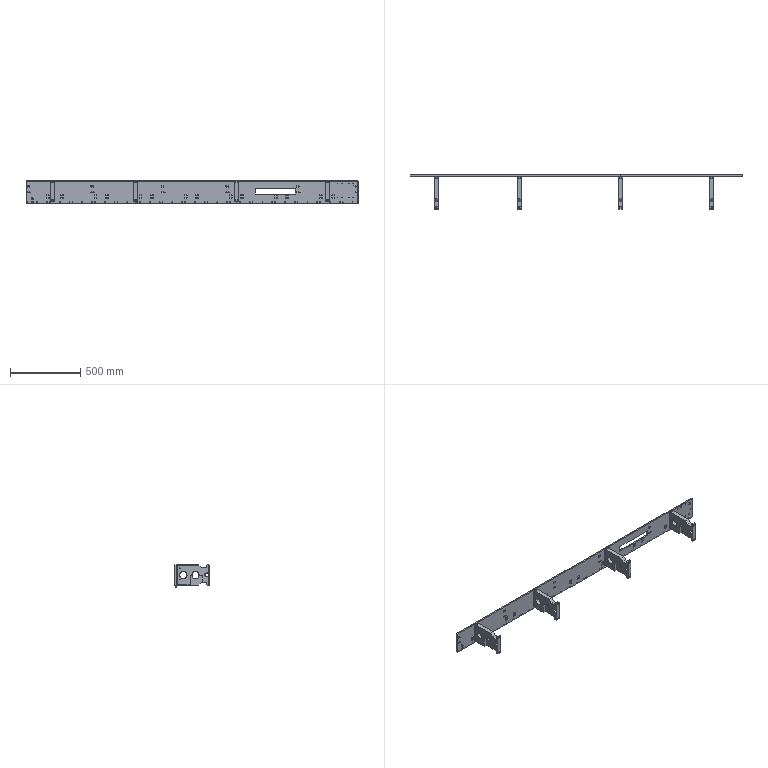Part | NX | 15 solids | 1566 faces | box 2359 x 243 x 161.5 mm | volume 6358915 mm3 | cylinder 654 | cone 542 | plane 370 | commonest cylinder face diameters 5 x268 4 x98 7 x64 2.5 x48 5.5 x44 10 x40